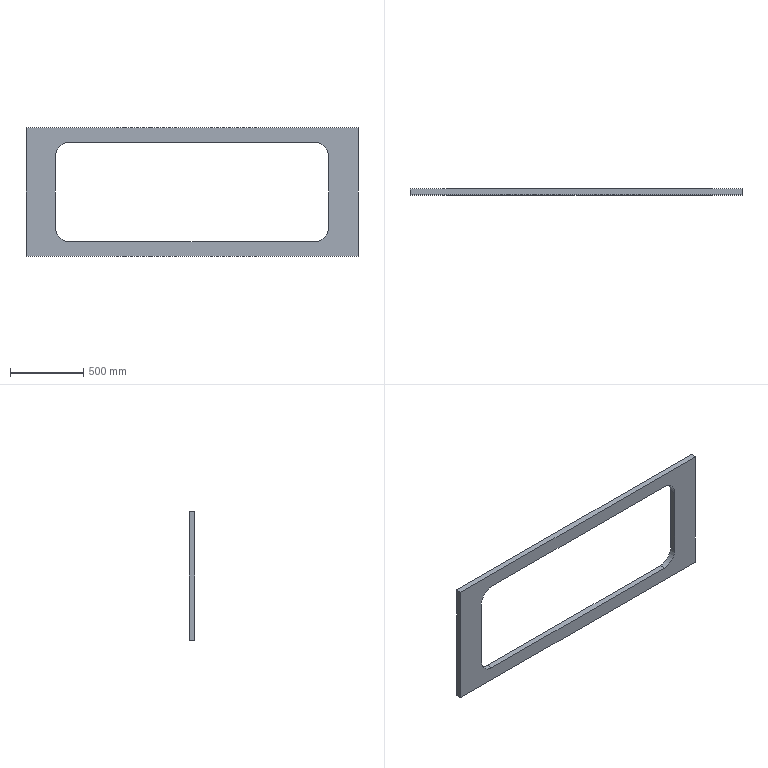Part | SolidWorks | features Cut 1, Extrusion 1, Fillet 1 | 1 solid | 14 faces | box 2266 x 40 x 880 mm | volume 29351363 mm3 | plane 10 | cylinder 4 | commonest cylinder face diameters 200 x4
STEP:
#1=CARTESIAN_POINT('',(1133.,0.,440.));
#2=VERTEX_POINT('',#1);
#3=CARTESIAN_POINT('',(1133.,0.,-440.));
#4=VERTEX_POINT('',#3);
#5=CARTESIAN_POINT('',(1133.,0.,440.));
#6=DIRECTION('',(0.,0.,-1.));
#7=VECTOR('',#6,1000.);
#8=LINE('',#5,#7);
#9=EDGE_CURVE('',#2,#4,#8,.T.);
#10=ORIENTED_EDGE('',*,*,#9,.T.);
#11=CARTESIAN_POINT('',(1133.,40.,-440.));
#12=VERTEX_POINT('',#11);
#13=CARTESIAN_POINT('',(1133.,40.,-440.));
#14=DIRECTION('',(0.,-1.,0.));
#15=VECTOR('',#14,1000.);
#16=LINE('',#13,#15);
#17=EDGE_CURVE('',#12,#4,#16,.T.);
#18=ORIENTED_EDGE('',*,*,#17,.F.);
#19=CARTESIAN_POINT('',(1133.,40.,440.));
#20=VERTEX_POINT('',#19);
#21=CARTESIAN_POINT('',(1133.,40.,440.));
#22=DIRECTION('',(0.,0.,-1.));
#23=VECTOR('',#22,1000.);
#24=LINE('',#21,#23);
#25=EDGE_CURVE('',#20,#12,#24,.T.);
#26=ORIENTED_EDGE('',*,*,#25,.F.);
#27=CARTESIAN_POINT('',(1133.,40.,440.));
#28=DIRECTION('',(0.,-1.,0.));
#29=VECTOR('',#28,1000.);
#30=LINE('',#27,#29);
#31=EDGE_CURVE('',#20,#2,#30,.T.);
#32=ORIENTED_EDGE('',*,*,#31,.T.);
#33=EDGE_LOOP('',(#10,#18,#26,#32));
#34=FACE_OUTER_BOUND('',#33,.T.);
#35=CARTESIAN_POINT('',(1133.,40.,440.));
#36=DIRECTION('',(-1.,0.,0.));
#37=DIRECTION('',(0.,0.,1.));
#38=AXIS2_PLACEMENT_3D('',#35,#36,#37);
#39=PLANE('',#38);
#40=ADVANCED_FACE('',(#34),#39,.F.);
#41=CARTESIAN_POINT('',(-1133.,0.,-440.));
#42=VERTEX_POINT('',#41);
#43=CARTESIAN_POINT('',(-1133.,0.,-440.));
#44=DIRECTION('',(-1.,0.,0.));
#45=VECTOR('',#44,1000.);
#46=LINE('',#43,#45);
#47=EDGE_CURVE('',#4,#42,#46,.T.);
#48=ORIENTED_EDGE('',*,*,#47,.T.);
#49=CARTESIAN_POINT('',(-1133.,40.,-440.));
#50=VERTEX_POINT('',#49);
#51=CARTESIAN_POINT('',(-1133.,40.,-440.));
#52=DIRECTION('',(0.,-1.,0.));
#53=VECTOR('',#52,1000.);
#54=LINE('',#51,#53);
#55=EDGE_CURVE('',#50,#42,#54,.T.);
#56=ORIENTED_EDGE('',*,*,#55,.F.);
#57=CARTESIAN_POINT('',(-1133.,40.,-440.));
#58=DIRECTION('',(-1.,0.,0.));
#59=VECTOR('',#58,1000.);
#60=LINE('',#57,#59);
#61=EDGE_CURVE('',#12,#50,#60,.T.);
#62=ORIENTED_EDGE('',*,*,#61,.F.);
#63=ORIENTED_EDGE('',*,*,#17,.T.);
#64=EDGE_LOOP('',(#48,#56,#62,#63));
#65=FACE_OUTER_BOUND('',#64,.T.);
#66=CARTESIAN_POINT('',(-1133.,40.,-440.));
#67=DIRECTION('',(0.,0.,1.));
#68=DIRECTION('',(1.,0.,0.));
#69=AXIS2_PLACEMENT_3D('',#66,#67,#68);
#70=PLANE('',#69);
#71=ADVANCED_FACE('',(#65),#70,.F.);
#72=CARTESIAN_POINT('',(-1133.,0.,440.));
#73=VERTEX_POINT('',#72);
#74=CARTESIAN_POINT('',(-1133.,0.,440.));
#75=DIRECTION('',(0.,0.,1.));
#76=VECTOR('',#75,1000.);
#77=LINE('',#74,#76);
#78=EDGE_CURVE('',#42,#73,#77,.T.);
#79=ORIENTED_EDGE('',*,*,#78,.T.);
#80=CARTESIAN_POINT('',(-1133.,40.,440.));
#81=VERTEX_POINT('',#80);
#82=CARTESIAN_POINT('',(-1133.,40.,440.));
#83=DIRECTION('',(0.,-1.,0.));
#84=VECTOR('',#83,1000.);
#85=LINE('',#82,#84);
#86=EDGE_CURVE('',#81,#73,#85,.T.);
#87=ORIENTED_EDGE('',*,*,#86,.F.);
#88=CARTESIAN_POINT('',(-1133.,40.,440.));
#89=DIRECTION('',(0.,0.,1.));
#90=VECTOR('',#89,1000.);
#91=LINE('',#88,#90);
#92=EDGE_CURVE('',#50,#81,#91,.T.);
#93=ORIENTED_EDGE('',*,*,#92,.F.);
#94=ORIENTED_EDGE('',*,*,#55,.T.);
#95=EDGE_LOOP('',(#79,#87,#93,#94));
#96=FACE_OUTER_BOUND('',#95,.T.);
#97=CARTESIAN_POINT('',(-1133.,40.,440.));
#98=DIRECTION('',(1.,0.,0.));
#99=DIRECTION('',(0.,0.,-1.));
#100=AXIS2_PLACEMENT_3D('',#97,#98,#99);
#101=PLANE('',#100);
#102=ADVANCED_FACE('',(#96),#101,.F.);
#103=CARTESIAN_POINT('',(-1133.,0.,440.));
#104=DIRECTION('',(1.,0.,0.));
#105=VECTOR('',#104,1000.);
#106=LINE('',#103,#105);
#107=EDGE_CURVE('',#73,#2,#106,.T.);
#108=ORIENTED_EDGE('',*,*,#107,.T.);
#109=ORIENTED_EDGE('',*,*,#31,.F.);
#110=CARTESIAN_POINT('',(-1133.,40.,440.));
#111=DIRECTION('',(1.,0.,0.));
#112=VECTOR('',#111,1000.);
#113=LINE('',#110,#112);
#114=EDGE_CURVE('',#81,#20,#113,.T.);
#115=ORIENTED_EDGE('',*,*,#114,.F.);
#116=ORIENTED_EDGE('',*,*,#86,.T.);
#117=EDGE_LOOP('',(#108,#109,#115,#116));
#118=FACE_OUTER_BOUND('',#117,.T.);
#119=CARTESIAN_POINT('',(-1133.,40.,440.));
#120=DIRECTION('',(0.,0.,-1.));
#121=DIRECTION('',(-1.,0.,0.));
#122=AXIS2_PLACEMENT_3D('',#119,#120,#121);
#123=PLANE('',#122);
#124=ADVANCED_FACE('',(#118),#123,.F.);
#125=CARTESIAN_POINT('',(-933.,40.,240.));
#126=VERTEX_POINT('',#125);
#127=CARTESIAN_POINT('',(-933.,40.,-240.));
#128=VERTEX_POINT('',#127);
#129=CARTESIAN_POINT('',(-933.,40.,340.));
#130=DIRECTION('',(0.,0.,-1.));
#131=VECTOR('',#130,1000.);
#132=LINE('',#129,#131);
#133=EDGE_CURVE('',#126,#128,#132,.T.);
#134=ORIENTED_EDGE('',*,*,#133,.T.);
#135=CARTESIAN_POINT('',(-833.,40.,-340.));
#136=VERTEX_POINT('',#135);
#137=CARTESIAN_POINT('',(-833.,40.,-240.));
#138=DIRECTION('',(0.,-1.,0.));
#139=DIRECTION('',(0.,0.,-1.));
#140=AXIS2_PLACEMENT_3D('',#137,#138,#139);
#141=CIRCLE('',#140,100.);
#142=EDGE_CURVE('',#128,#136,#141,.T.);
#143=ORIENTED_EDGE('',*,*,#142,.T.);
#144=CARTESIAN_POINT('',(833.,40.,-340.));
#145=VERTEX_POINT('',#144);
#146=CARTESIAN_POINT('',(-933.,40.,-340.));
#147=DIRECTION('',(1.,0.,0.));
#148=VECTOR('',#147,1000.);
#149=LINE('',#146,#148);
#150=EDGE_CURVE('',#136,#145,#149,.T.);
#151=ORIENTED_EDGE('',*,*,#150,.T.);
#152=CARTESIAN_POINT('',(933.,40.,-240.));
#153=VERTEX_POINT('',#152);
#154=CARTESIAN_POINT('',(833.,40.,-240.));
#155=DIRECTION('',(0.,-1.,0.));
#156=DIRECTION('',(0.,0.,-1.));
#157=AXIS2_PLACEMENT_3D('',#154,#155,#156);
#158=CIRCLE('',#157,100.);
#159=EDGE_CURVE('',#145,#153,#158,.T.);
#160=ORIENTED_EDGE('',*,*,#159,.T.);
#161=CARTESIAN_POINT('',(933.,40.,240.));
#162=VERTEX_POINT('',#161);
#163=CARTESIAN_POINT('',(933.,40.,340.));
#164=DIRECTION('',(0.,0.,1.));
#165=VECTOR('',#164,1000.);
#166=LINE('',#163,#165);
#167=EDGE_CURVE('',#153,#162,#166,.T.);
#168=ORIENTED_EDGE('',*,*,#167,.T.);
#169=CARTESIAN_POINT('',(833.,40.,340.));
#170=VERTEX_POINT('',#169);
#171=CARTESIAN_POINT('',(833.,40.,240.));
#172=DIRECTION('',(0.,-1.,0.));
#173=DIRECTION('',(0.,0.,-1.));
#174=AXIS2_PLACEMENT_3D('',#171,#172,#173);
#175=CIRCLE('',#174,100.);
#176=EDGE_CURVE('',#162,#170,#175,.T.);
#177=ORIENTED_EDGE('',*,*,#176,.T.);
#178=CARTESIAN_POINT('',(-833.,40.,340.));
#179=VERTEX_POINT('',#178);
#180=CARTESIAN_POINT('',(-933.,40.,340.));
#181=DIRECTION('',(-1.,0.,0.));
#182=VECTOR('',#181,1000.);
#183=LINE('',#180,#182);
#184=EDGE_CURVE('',#170,#179,#183,.T.);
#185=ORIENTED_EDGE('',*,*,#184,.T.);
#186=CARTESIAN_POINT('',(-833.,40.,240.));
#187=DIRECTION('',(0.,-1.,0.));
#188=DIRECTION('',(0.,0.,-1.));
#189=AXIS2_PLACEMENT_3D('',#186,#187,#188);
#190=CIRCLE('',#189,100.);
#191=EDGE_CURVE('',#179,#126,#190,.T.);
#192=ORIENTED_EDGE('',*,*,#191,.T.);
#193=EDGE_LOOP('',(#134,#143,#151,#160,#168,#177,#185,#192));
#194=FACE_BOUND('',#193,.T.);
#195=ORIENTED_EDGE('',*,*,#25,.T.);
#196=ORIENTED_EDGE('',*,*,#61,.T.);
#197=ORIENTED_EDGE('',*,*,#92,.T.);
#198=ORIENTED_EDGE('',*,*,#114,.T.);
#199=EDGE_LOOP('',(#195,#196,#197,#198));
#200=FACE_OUTER_BOUND('',#199,.T.);
#201=CARTESIAN_POINT('',(0.,40.,0.));
#202=DIRECTION('',(0.,-1.,0.));
#203=DIRECTION('',(0.,0.,-1.));
#204=AXIS2_PLACEMENT_3D('',#201,#202,#203);
#205=PLANE('',#204);
#206=ADVANCED_FACE('',(#194,#200),#205,.F.);
#207=CARTESIAN_POINT('',(933.,0.,-240.));
#208=VERTEX_POINT('',#207);
#209=CARTESIAN_POINT('',(933.,0.,240.));
#210=VERTEX_POINT('',#209);
#211=CARTESIAN_POINT('',(933.,0.,340.));
#212=DIRECTION('',(0.,0.,1.));
#213=VECTOR('',#212,1000.);
#214=LINE('',#211,#213);
#215=EDGE_CURVE('',#208,#210,#214,.T.);
#216=ORIENTED_EDGE('',*,*,#215,.F.);
#217=CARTESIAN_POINT('',(833.,0.,-340.));
#218=VERTEX_POINT('',#217);
#219=CARTESIAN_POINT('',(833.,0.,-240.));
#220=DIRECTION('',(0.,1.,0.));
#221=DIRECTION('',(0.,0.,-1.));
#222=AXIS2_PLACEMENT_3D('',#219,#220,#221);
#223=CIRCLE('',#222,100.);
#224=EDGE_CURVE('',#208,#218,#223,.T.);
#225=ORIENTED_EDGE('',*,*,#224,.T.);
#226=CARTESIAN_POINT('',(-833.,0.,-340.));
#227=VERTEX_POINT('',#226);
#228=CARTESIAN_POINT('',(-933.,0.,-340.));
#229=DIRECTION('',(1.,0.,0.));
#230=VECTOR('',#229,1000.);
#231=LINE('',#228,#230);
#232=EDGE_CURVE('',#227,#218,#231,.T.);
#233=ORIENTED_EDGE('',*,*,#232,.F.);
#234=CARTESIAN_POINT('',(-933.,0.,-240.));
#235=VERTEX_POINT('',#234);
#236=CARTESIAN_POINT('',(-833.,0.,-240.));
#237=DIRECTION('',(0.,1.,0.));
#238=DIRECTION('',(0.,0.,-1.));
#239=AXIS2_PLACEMENT_3D('',#236,#237,#238);
#240=CIRCLE('',#239,100.);
#241=EDGE_CURVE('',#227,#235,#240,.T.);
#242=ORIENTED_EDGE('',*,*,#241,.T.);
#243=CARTESIAN_POINT('',(-933.,0.,240.));
#244=VERTEX_POINT('',#243);
#245=CARTESIAN_POINT('',(-933.,0.,340.));
#246=DIRECTION('',(0.,0.,-1.));
#247=VECTOR('',#246,1000.);
#248=LINE('',#245,#247);
#249=EDGE_CURVE('',#244,#235,#248,.T.);
#250=ORIENTED_EDGE('',*,*,#249,.F.);
#251=CARTESIAN_POINT('',(-833.,0.,340.));
#252=VERTEX_POINT('',#251);
#253=CARTESIAN_POINT('',(-833.,0.,240.));
#254=DIRECTION('',(0.,1.,0.));
#255=DIRECTION('',(0.,0.,-1.));
#256=AXIS2_PLACEMENT_3D('',#253,#254,#255);
#257=CIRCLE('',#256,100.);
#258=EDGE_CURVE('',#244,#252,#257,.T.);
#259=ORIENTED_EDGE('',*,*,#258,.T.);
#260=CARTESIAN_POINT('',(833.,0.,340.));
#261=VERTEX_POINT('',#260);
#262=CARTESIAN_POINT('',(-933.,0.,340.));
#263=DIRECTION('',(-1.,0.,0.));
#264=VECTOR('',#263,1000.);
#265=LINE('',#262,#264);
#266=EDGE_CURVE('',#261,#252,#265,.T.);
#267=ORIENTED_EDGE('',*,*,#266,.F.);
#268=CARTESIAN_POINT('',(833.,0.,240.));
#269=DIRECTION('',(0.,1.,0.));
#270=DIRECTION('',(0.,0.,-1.));
#271=AXIS2_PLACEMENT_3D('',#268,#269,#270);
#272=CIRCLE('',#271,100.);
#273=EDGE_CURVE('',#261,#210,#272,.T.);
#274=ORIENTED_EDGE('',*,*,#273,.T.);
#275=EDGE_LOOP('',(#216,#225,#233,#242,#250,#259,#267,#274));
#276=FACE_BOUND('',#275,.T.);
#277=ORIENTED_EDGE('',*,*,#9,.F.);
#278=ORIENTED_EDGE('',*,*,#107,.F.);
#279=ORIENTED_EDGE('',*,*,#78,.F.);
#280=ORIENTED_EDGE('',*,*,#47,.F.);
#281=EDGE_LOOP('',(#277,#278,#279,#280));
#282=FACE_OUTER_BOUND('',#281,.T.);
#283=CARTESIAN_POINT('',(0.,0.,0.));
#284=DIRECTION('',(0.,-1.,0.));
#285=DIRECTION('',(0.,0.,-1.));
#286=AXIS2_PLACEMENT_3D('',#283,#284,#285);
#287=PLANE('',#286);
#288=ADVANCED_FACE('',(#276,#282),#287,.T.);
#289=ORIENTED_EDGE('',*,*,#167,.F.);
#290=CARTESIAN_POINT('',(933.,0.,-240.));
#291=DIRECTION('',(0.,-1.,0.));
#292=VECTOR('',#291,1000.);
#293=LINE('',#290,#292);
#294=EDGE_CURVE('',#153,#208,#293,.T.);
#295=ORIENTED_EDGE('',*,*,#294,.T.);
#296=ORIENTED_EDGE('',*,*,#215,.T.);
#297=CARTESIAN_POINT('',(933.,40.,240.));
#298=DIRECTION('',(0.,1.,0.));
#299=VECTOR('',#298,1000.);
#300=LINE('',#297,#299);
#301=EDGE_CURVE('',#210,#162,#300,.T.);
#302=ORIENTED_EDGE('',*,*,#301,.T.);
#303=EDGE_LOOP('',(#289,#295,#296,#302));
#304=FACE_OUTER_BOUND('',#303,.T.);
#305=CARTESIAN_POINT('',(933.,40.,340.));
#306=DIRECTION('',(1.,0.,0.));
#307=DIRECTION('',(0.,0.,-1.));
#308=AXIS2_PLACEMENT_3D('',#305,#306,#307);
#309=PLANE('',#308);
#310=ADVANCED_FACE('',(#304),#309,.F.);
#311=ORIENTED_EDGE('',*,*,#150,.F.);
#312=CARTESIAN_POINT('',(-833.,0.,-340.));
#313=DIRECTION('',(0.,-1.,0.));
#314=VECTOR('',#313,1000.);
#315=LINE('',#312,#314);
#316=EDGE_CURVE('',#136,#227,#315,.T.);
#317=ORIENTED_EDGE('',*,*,#316,.T.);
#318=ORIENTED_EDGE('',*,*,#232,.T.);
#319=CARTESIAN_POINT('',(833.,40.,-340.));
#320=DIRECTION('',(0.,1.,0.));
#321=VECTOR('',#320,1000.);
#322=LINE('',#319,#321);
#323=EDGE_CURVE('',#218,#145,#322,.T.);
#324=ORIENTED_EDGE('',*,*,#323,.T.);
#325=EDGE_LOOP('',(#311,#317,#318,#324));
#326=FACE_OUTER_BOUND('',#325,.T.);
#327=CARTESIAN_POINT('',(-933.,40.,-340.));
#328=DIRECTION('',(0.,0.,-1.));
#329=DIRECTION('',(-1.,0.,0.));
#330=AXIS2_PLACEMENT_3D('',#327,#328,#329);
#331=PLANE('',#330);
#332=ADVANCED_FACE('',(#326),#331,.F.);
#333=ORIENTED_EDGE('',*,*,#249,.T.);
#334=CARTESIAN_POINT('',(-933.,40.,-240.));
#335=DIRECTION('',(0.,1.,0.));
#336=VECTOR('',#335,1000.);
#337=LINE('',#334,#336);
#338=EDGE_CURVE('',#235,#128,#337,.T.);
#339=ORIENTED_EDGE('',*,*,#338,.T.);
#340=ORIENTED_EDGE('',*,*,#133,.F.);
#341=CARTESIAN_POINT('',(-933.,0.,240.));
#342=DIRECTION('',(0.,-1.,0.));
#343=VECTOR('',#342,1000.);
#344=LINE('',#341,#343);
#345=EDGE_CURVE('',#126,#244,#344,.T.);
#346=ORIENTED_EDGE('',*,*,#345,.T.);
#347=EDGE_LOOP('',(#333,#339,#340,#346));
#348=FACE_OUTER_BOUND('',#347,.T.);
#349=CARTESIAN_POINT('',(-933.,40.,340.));
#350=DIRECTION('',(-1.,0.,0.));
#351=DIRECTION('',(0.,0.,1.));
#352=AXIS2_PLACEMENT_3D('',#349,#350,#351);
#353=PLANE('',#352);
#354=ADVANCED_FACE('',(#348),#353,.F.);
#355=ORIENTED_EDGE('',*,*,#266,.T.);
#356=CARTESIAN_POINT('',(-833.,40.,340.));
#357=DIRECTION('',(0.,1.,0.));
#358=VECTOR('',#357,1000.);
#359=LINE('',#356,#358);
#360=EDGE_CURVE('',#252,#179,#359,.T.);
#361=ORIENTED_EDGE('',*,*,#360,.T.);
#362=ORIENTED_EDGE('',*,*,#184,.F.);
#363=CARTESIAN_POINT('',(833.,0.,340.));
#364=DIRECTION('',(0.,-1.,0.));
#365=VECTOR('',#364,1000.);
#366=LINE('',#363,#365);
#367=EDGE_CURVE('',#170,#261,#366,.T.);
#368=ORIENTED_EDGE('',*,*,#367,.T.);
#369=EDGE_LOOP('',(#355,#361,#362,#368));
#370=FACE_OUTER_BOUND('',#369,.T.);
#371=CARTESIAN_POINT('',(-933.,40.,340.));
#372=DIRECTION('',(0.,0.,1.));
#373=DIRECTION('',(1.,0.,0.));
#374=AXIS2_PLACEMENT_3D('',#371,#372,#373);
#375=PLANE('',#374);
#376=ADVANCED_FACE('',(#370),#375,.F.);
#377=ORIENTED_EDGE('',*,*,#142,.F.);
#378=ORIENTED_EDGE('',*,*,#338,.F.);
#379=ORIENTED_EDGE('',*,*,#241,.F.);
#380=ORIENTED_EDGE('',*,*,#316,.F.);
#381=EDGE_LOOP('',(#377,#378,#379,#380));
#382=FACE_OUTER_BOUND('',#381,.T.);
#383=CARTESIAN_POINT('',(-833.,40.,-240.));
#384=DIRECTION('',(0.,1.,0.));
#385=DIRECTION('',(0.,0.,1.));
#386=AXIS2_PLACEMENT_3D('',#383,#384,#385);
#387=CYLINDRICAL_SURFACE('',#386,100.);
#388=ADVANCED_FACE('',(#382),#387,.F.);
#389=ORIENTED_EDGE('',*,*,#191,.F.);
#390=ORIENTED_EDGE('',*,*,#360,.F.);
#391=ORIENTED_EDGE('',*,*,#258,.F.);
#392=ORIENTED_EDGE('',*,*,#345,.F.);
#393=EDGE_LOOP('',(#389,#390,#391,#392));
#394=FACE_OUTER_BOUND('',#393,.T.);
#395=CARTESIAN_POINT('',(-833.,40.,240.));
#396=DIRECTION('',(0.,1.,0.));
#397=DIRECTION('',(0.,0.,1.));
#398=AXIS2_PLACEMENT_3D('',#395,#396,#397);
#399=CYLINDRICAL_SURFACE('',#398,100.);
#400=ADVANCED_FACE('',(#394),#399,.F.);
#401=ORIENTED_EDGE('',*,*,#159,.F.);
#402=ORIENTED_EDGE('',*,*,#323,.F.);
#403=ORIENTED_EDGE('',*,*,#224,.F.);
#404=ORIENTED_EDGE('',*,*,#294,.F.);
#405=EDGE_LOOP('',(#401,#402,#403,#404));
#406=FACE_OUTER_BOUND('',#405,.T.);
#407=CARTESIAN_POINT('',(833.,40.,-240.));
#408=DIRECTION('',(0.,1.,0.));
#409=DIRECTION('',(0.,0.,1.));
#410=AXIS2_PLACEMENT_3D('',#407,#408,#409);
#411=CYLINDRICAL_SURFACE('',#410,100.);
#412=ADVANCED_FACE('',(#406),#411,.F.);
#413=ORIENTED_EDGE('',*,*,#176,.F.);
#414=ORIENTED_EDGE('',*,*,#301,.F.);
#415=ORIENTED_EDGE('',*,*,#273,.F.);
#416=ORIENTED_EDGE('',*,*,#367,.F.);
#417=EDGE_LOOP('',(#413,#414,#415,#416));
#418=FACE_OUTER_BOUND('',#417,.T.);
#419=CARTESIAN_POINT('',(833.,40.,240.));
#420=DIRECTION('',(0.,1.,0.));
#421=DIRECTION('',(0.,0.,1.));
#422=AXIS2_PLACEMENT_3D('',#419,#420,#421);
#423=CYLINDRICAL_SURFACE('',#422,100.);
#424=ADVANCED_FACE('',(#418),#423,.F.);
#425=CLOSED_SHELL('',(#40,#71,#102,#124,#206,#288,#310,#332,#354,#376,#388,#400,#412,#424));
#426=MANIFOLD_SOLID_BREP('',#425);
#427=CARTESIAN_POINT('',(0.,0.,0.));
#428=DIRECTION('',(0.,0.,1.));
#429=DIRECTION('',(1.,0.,0.));
#430=AXIS2_PLACEMENT_3D('',#427,#428,#429);
#431=(LENGTH_UNIT()NAMED_UNIT(*)SI_UNIT(.MILLI.,.METRE.));
#432=UNCERTAINTY_MEASURE_WITH_UNIT(LENGTH_MEASURE(0.00001),#431,'','');
#433=(NAMED_UNIT(*)PLANE_ANGLE_UNIT()SI_UNIT($,.RADIAN.));
#434=(NAMED_UNIT(*)SI_UNIT($,.STERADIAN.)SOLID_ANGLE_UNIT());
#435=(GEOMETRIC_REPRESENTATION_CONTEXT(3)GLOBAL_UNCERTAINTY_ASSIGNED_CONTEXT((#432))GLOBAL_UNIT_ASSIGNED_CONTEXT((#431,#433,#434))REPRESENTATION_CONTEXT('',''));
#436=ADVANCED_BREP_SHAPE_REPRESENTATION('',(#426,#430),#435);